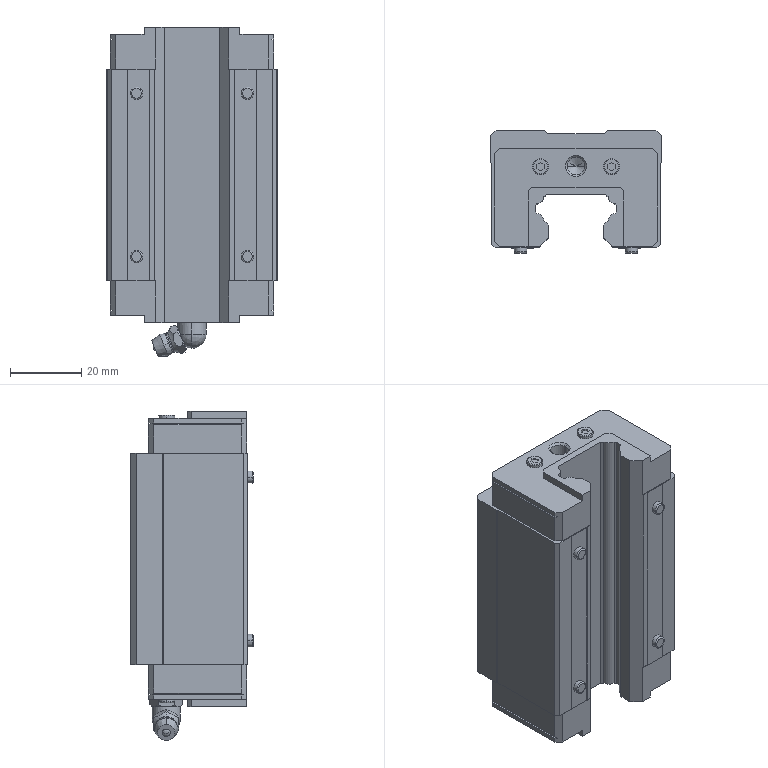Part | SolidWorks | features BaseBody 2 | 2 solids | 381 faces | box 48 x 34.5 x 92.7 mm | volume 95932 mm3 | plane 155 | cylinder 154 | cone 33 | torus 22 | spline 11 | sphere 6 | commonest cylinder face diameters 6 x66 4.701 x60 3.518 x8 4.5 x8 4.917 x4 4.96 x4